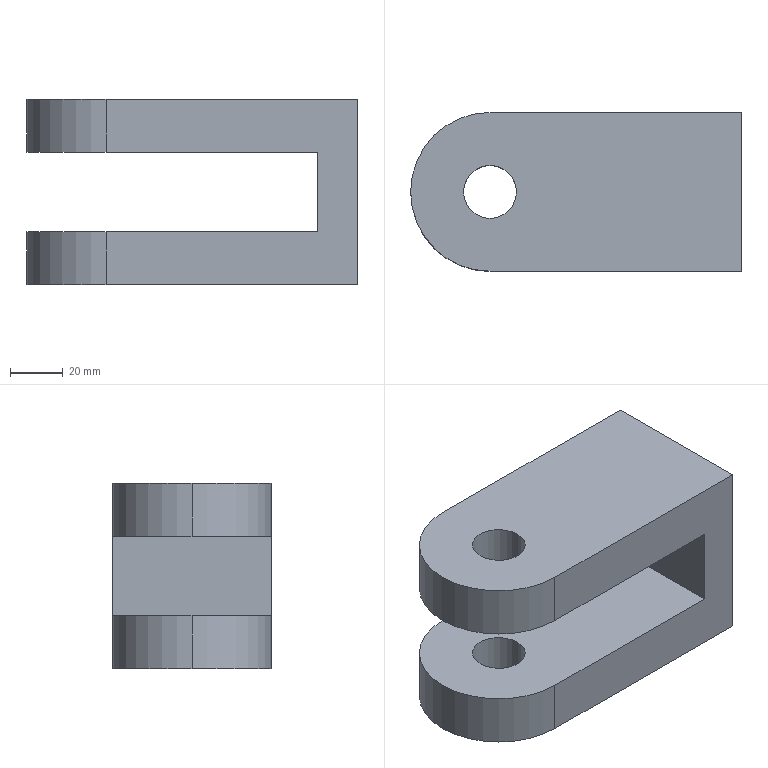Part | SolidWorks | features ICE 2, Extrusion 1, MirrorSolid 1 | 1 solid | 16 faces | box 125 x 60 x 70 mm | volume 298982 mm3 | cylinder 8 | plane 8 | commonest cylinder face diameters 20 x4 60 x4
STEP:
#1=CARTESIAN_POINT('',(-50.,0.,-50.));
#2=VERTEX_POINT('',#1);
#3=CARTESIAN_POINT('',(-30.,0.,-50.));
#4=VERTEX_POINT('',#3);
#5=CARTESIAN_POINT('',(-40.,0.,-50.));
#6=DIRECTION('',(0.,0.,-1.));
#7=DIRECTION('',(-1.,0.,0.));
#8=AXIS2_PLACEMENT_3D('',#5,#6,#7);
#9=CIRCLE('',#8,10.);
#10=EDGE_CURVE('',#2,#4,#9,.T.);
#11=ORIENTED_EDGE('',*,*,#10,.T.);
#12=CARTESIAN_POINT('',(-30.,0.,-30.));
#13=VERTEX_POINT('',#12);
#14=CARTESIAN_POINT('',(-30.,0.,-50.));
#15=DIRECTION('',(0.,0.,1.));
#16=VECTOR('',#15,1000.);
#17=LINE('',#14,#16);
#18=EDGE_CURVE('',#4,#13,#17,.T.);
#19=ORIENTED_EDGE('',*,*,#18,.T.);
#20=CARTESIAN_POINT('',(-50.,0.,-30.));
#21=VERTEX_POINT('',#20);
#22=CARTESIAN_POINT('',(-40.,0.,-30.));
#23=DIRECTION('',(0.,0.,-1.));
#24=DIRECTION('',(-1.,0.,0.));
#25=AXIS2_PLACEMENT_3D('',#22,#23,#24);
#26=CIRCLE('',#25,10.);
#27=EDGE_CURVE('',#21,#13,#26,.T.);
#28=ORIENTED_EDGE('',*,*,#27,.F.);
#29=CARTESIAN_POINT('',(-50.,0.,-50.));
#30=DIRECTION('',(0.,0.,1.));
#31=VECTOR('',#30,1000.);
#32=LINE('',#29,#31);
#33=EDGE_CURVE('',#2,#21,#32,.T.);
#34=ORIENTED_EDGE('',*,*,#33,.F.);
#35=EDGE_LOOP('',(#11,#19,#28,#34));
#36=FACE_OUTER_BOUND('',#35,.T.);
#37=CARTESIAN_POINT('',(-40.,0.,-50.));
#38=DIRECTION('',(0.,0.,1.));
#39=DIRECTION('',(-1.,0.,0.));
#40=AXIS2_PLACEMENT_3D('',#37,#38,#39);
#41=CYLINDRICAL_SURFACE('',#40,10.);
#42=ADVANCED_FACE('',(#36),#41,.F.);
#43=CARTESIAN_POINT('',(-40.,30.,-50.));
#44=VERTEX_POINT('',#43);
#45=CARTESIAN_POINT('',(-70.,0.,-50.));
#46=VERTEX_POINT('',#45);
#47=CARTESIAN_POINT('',(-40.,0.,-50.));
#48=DIRECTION('',(0.,0.,1.));
#49=DIRECTION('',(1.,0.,0.));
#50=AXIS2_PLACEMENT_3D('',#47,#48,#49);
#51=CIRCLE('',#50,30.);
#52=EDGE_CURVE('',#44,#46,#51,.T.);
#53=ORIENTED_EDGE('',*,*,#52,.T.);
#54=CARTESIAN_POINT('',(-70.,0.,-30.));
#55=VERTEX_POINT('',#54);
#56=CARTESIAN_POINT('',(-70.,0.,-50.));
#57=DIRECTION('',(0.,0.,1.));
#58=VECTOR('',#57,1000.);
#59=LINE('',#56,#58);
#60=EDGE_CURVE('',#46,#55,#59,.T.);
#61=ORIENTED_EDGE('',*,*,#60,.T.);
#62=CARTESIAN_POINT('',(-40.,30.,-30.));
#63=VERTEX_POINT('',#62);
#64=CARTESIAN_POINT('',(-40.,0.,-30.));
#65=DIRECTION('',(0.,0.,1.));
#66=DIRECTION('',(1.,0.,0.));
#67=AXIS2_PLACEMENT_3D('',#64,#65,#66);
#68=CIRCLE('',#67,30.);
#69=EDGE_CURVE('',#63,#55,#68,.T.);
#70=ORIENTED_EDGE('',*,*,#69,.F.);
#71=CARTESIAN_POINT('',(-40.,30.,-50.));
#72=DIRECTION('',(0.,0.,1.));
#73=VECTOR('',#72,1000.);
#74=LINE('',#71,#73);
#75=EDGE_CURVE('',#44,#63,#74,.T.);
#76=ORIENTED_EDGE('',*,*,#75,.F.);
#77=EDGE_LOOP('',(#53,#61,#70,#76));
#78=FACE_OUTER_BOUND('',#77,.T.);
#79=CARTESIAN_POINT('',(-40.,0.,-50.));
#80=DIRECTION('',(0.,0.,1.));
#81=DIRECTION('',(-1.,0.,0.));
#82=AXIS2_PLACEMENT_3D('',#79,#80,#81);
#83=CYLINDRICAL_SURFACE('',#82,30.);
#84=ADVANCED_FACE('',(#78),#83,.T.);
#85=CARTESIAN_POINT('',(-30.,0.,20.));
#86=VERTEX_POINT('',#85);
#87=CARTESIAN_POINT('',(-50.,0.,20.));
#88=VERTEX_POINT('',#87);
#89=CARTESIAN_POINT('',(-40.,0.,20.));
#90=DIRECTION('',(0.,0.,-1.));
#91=DIRECTION('',(-1.,0.,0.));
#92=AXIS2_PLACEMENT_3D('',#89,#90,#91);
#93=CIRCLE('',#92,10.);
#94=EDGE_CURVE('',#86,#88,#93,.T.);
#95=ORIENTED_EDGE('',*,*,#94,.F.);
#96=CARTESIAN_POINT('',(-30.,0.,0.));
#97=VERTEX_POINT('',#96);
#98=CARTESIAN_POINT('',(-30.,0.,20.));
#99=DIRECTION('',(0.,0.,-1.));
#100=VECTOR('',#99,1000.);
#101=LINE('',#98,#100);
#102=EDGE_CURVE('',#86,#97,#101,.T.);
#103=ORIENTED_EDGE('',*,*,#102,.T.);
#104=CARTESIAN_POINT('',(-50.,0.,0.));
#105=VERTEX_POINT('',#104);
#106=CARTESIAN_POINT('',(-40.,0.,0.));
#107=DIRECTION('',(0.,0.,-1.));
#108=DIRECTION('',(-1.,0.,0.));
#109=AXIS2_PLACEMENT_3D('',#106,#107,#108);
#110=CIRCLE('',#109,10.);
#111=EDGE_CURVE('',#97,#105,#110,.T.);
#112=ORIENTED_EDGE('',*,*,#111,.T.);
#113=CARTESIAN_POINT('',(-50.,0.,20.));
#114=DIRECTION('',(0.,0.,-1.));
#115=VECTOR('',#114,1000.);
#116=LINE('',#113,#115);
#117=EDGE_CURVE('',#88,#105,#116,.T.);
#118=ORIENTED_EDGE('',*,*,#117,.F.);
#119=EDGE_LOOP('',(#95,#103,#112,#118));
#120=FACE_OUTER_BOUND('',#119,.T.);
#121=CARTESIAN_POINT('',(-40.,0.,20.));
#122=DIRECTION('',(0.,0.,-1.));
#123=DIRECTION('',(-1.,0.,0.));
#124=AXIS2_PLACEMENT_3D('',#121,#122,#123);
#125=CYLINDRICAL_SURFACE('',#124,10.);
#126=ADVANCED_FACE('',(#120),#125,.F.);
#127=CARTESIAN_POINT('',(-70.,0.,20.));
#128=VERTEX_POINT('',#127);
#129=CARTESIAN_POINT('',(-40.,-30.,20.));
#130=VERTEX_POINT('',#129);
#131=CARTESIAN_POINT('',(-40.,0.,20.));
#132=DIRECTION('',(0.,0.,1.));
#133=DIRECTION('',(1.,0.,0.));
#134=AXIS2_PLACEMENT_3D('',#131,#132,#133);
#135=CIRCLE('',#134,30.);
#136=EDGE_CURVE('',#128,#130,#135,.T.);
#137=ORIENTED_EDGE('',*,*,#136,.F.);
#138=CARTESIAN_POINT('',(-70.,0.,0.));
#139=VERTEX_POINT('',#138);
#140=CARTESIAN_POINT('',(-70.,0.,20.));
#141=DIRECTION('',(0.,0.,-1.));
#142=VECTOR('',#141,1000.);
#143=LINE('',#140,#142);
#144=EDGE_CURVE('',#128,#139,#143,.T.);
#145=ORIENTED_EDGE('',*,*,#144,.T.);
#146=CARTESIAN_POINT('',(-40.,-30.,0.));
#147=VERTEX_POINT('',#146);
#148=CARTESIAN_POINT('',(-40.,0.,0.));
#149=DIRECTION('',(0.,0.,1.));
#150=DIRECTION('',(1.,0.,0.));
#151=AXIS2_PLACEMENT_3D('',#148,#149,#150);
#152=CIRCLE('',#151,30.);
#153=EDGE_CURVE('',#139,#147,#152,.T.);
#154=ORIENTED_EDGE('',*,*,#153,.T.);
#155=CARTESIAN_POINT('',(-40.,-30.,20.));
#156=DIRECTION('',(0.,0.,-1.));
#157=VECTOR('',#156,1000.);
#158=LINE('',#155,#157);
#159=EDGE_CURVE('',#130,#147,#158,.T.);
#160=ORIENTED_EDGE('',*,*,#159,.F.);
#161=EDGE_LOOP('',(#137,#145,#154,#160));
#162=FACE_OUTER_BOUND('',#161,.T.);
#163=CARTESIAN_POINT('',(-40.,0.,20.));
#164=DIRECTION('',(0.,0.,-1.));
#165=DIRECTION('',(-1.,0.,0.));
#166=AXIS2_PLACEMENT_3D('',#163,#164,#165);
#167=CYLINDRICAL_SURFACE('',#166,30.);
#168=ADVANCED_FACE('',(#162),#167,.T.);
#169=CARTESIAN_POINT('',(40.,30.,0.));
#170=VERTEX_POINT('',#169);
#171=CARTESIAN_POINT('',(-40.,30.,0.));
#172=VERTEX_POINT('',#171);
#173=CARTESIAN_POINT('',(-40.,30.,0.));
#174=DIRECTION('',(-1.,0.,0.));
#175=VECTOR('',#174,1000.);
#176=LINE('',#173,#175);
#177=EDGE_CURVE('',#170,#172,#176,.T.);
#178=ORIENTED_EDGE('',*,*,#177,.T.);
#179=CARTESIAN_POINT('',(-40.,30.,20.));
#180=VERTEX_POINT('',#179);
#181=CARTESIAN_POINT('',(-40.,30.,20.));
#182=DIRECTION('',(0.,0.,-1.));
#183=VECTOR('',#182,1000.);
#184=LINE('',#181,#183);
#185=EDGE_CURVE('',#180,#172,#184,.T.);
#186=ORIENTED_EDGE('',*,*,#185,.F.);
#187=CARTESIAN_POINT('',(55.,30.,20.));
#188=VERTEX_POINT('',#187);
#189=CARTESIAN_POINT('',(-40.,30.,20.));
#190=DIRECTION('',(-1.,0.,0.));
#191=VECTOR('',#190,1000.);
#192=LINE('',#189,#191);
#193=EDGE_CURVE('',#188,#180,#192,.T.);
#194=ORIENTED_EDGE('',*,*,#193,.F.);
#195=CARTESIAN_POINT('',(55.,30.,-50.));
#196=VERTEX_POINT('',#195);
#197=CARTESIAN_POINT('',(55.,30.,20.));
#198=DIRECTION('',(0.,0.,1.));
#199=VECTOR('',#198,1000.);
#200=LINE('',#197,#199);
#201=EDGE_CURVE('',#196,#188,#200,.T.);
#202=ORIENTED_EDGE('',*,*,#201,.F.);
#203=CARTESIAN_POINT('',(-40.,30.,-50.));
#204=DIRECTION('',(-1.,0.,0.));
#205=VECTOR('',#204,1000.);
#206=LINE('',#203,#205);
#207=EDGE_CURVE('',#196,#44,#206,.T.);
#208=ORIENTED_EDGE('',*,*,#207,.T.);
#209=ORIENTED_EDGE('',*,*,#75,.T.);
#210=CARTESIAN_POINT('',(40.,30.,-30.));
#211=VERTEX_POINT('',#210);
#212=CARTESIAN_POINT('',(-40.,30.,-30.));
#213=DIRECTION('',(-1.,0.,0.));
#214=VECTOR('',#213,1000.);
#215=LINE('',#212,#214);
#216=EDGE_CURVE('',#211,#63,#215,.T.);
#217=ORIENTED_EDGE('',*,*,#216,.F.);
#218=CARTESIAN_POINT('',(40.,30.,20.));
#219=DIRECTION('',(0.,0.,1.));
#220=VECTOR('',#219,1000.);
#221=LINE('',#218,#220);
#222=EDGE_CURVE('',#211,#170,#221,.T.);
#223=ORIENTED_EDGE('',*,*,#222,.T.);
#224=EDGE_LOOP('',(#178,#186,#194,#202,#208,#209,#217,#223));
#225=FACE_OUTER_BOUND('',#224,.T.);
#226=CARTESIAN_POINT('',(-40.,30.,20.));
#227=DIRECTION('',(0.,-1.,0.));
#228=DIRECTION('',(0.,0.,-1.));
#229=AXIS2_PLACEMENT_3D('',#226,#227,#228);
#230=PLANE('',#229);
#231=ADVANCED_FACE('',(#225),#230,.F.);
#232=ORIENTED_EDGE('',*,*,#144,.F.);
#233=CARTESIAN_POINT('',(-40.,0.,20.));
#234=DIRECTION('',(0.,0.,1.));
#235=DIRECTION('',(1.,0.,0.));
#236=AXIS2_PLACEMENT_3D('',#233,#234,#235);
#237=CIRCLE('',#236,30.);
#238=EDGE_CURVE('',#180,#128,#237,.T.);
#239=ORIENTED_EDGE('',*,*,#238,.F.);
#240=ORIENTED_EDGE('',*,*,#185,.T.);
#241=CARTESIAN_POINT('',(-40.,0.,0.));
#242=DIRECTION('',(0.,0.,1.));
#243=DIRECTION('',(1.,0.,0.));
#244=AXIS2_PLACEMENT_3D('',#241,#242,#243);
#245=CIRCLE('',#244,30.);
#246=EDGE_CURVE('',#172,#139,#245,.T.);
#247=ORIENTED_EDGE('',*,*,#246,.T.);
#248=EDGE_LOOP('',(#232,#239,#240,#247));
#249=FACE_OUTER_BOUND('',#248,.T.);
#250=CARTESIAN_POINT('',(-40.,0.,20.));
#251=DIRECTION('',(0.,0.,-1.));
#252=DIRECTION('',(-1.,0.,0.));
#253=AXIS2_PLACEMENT_3D('',#250,#251,#252);
#254=CYLINDRICAL_SURFACE('',#253,30.);
#255=ADVANCED_FACE('',(#249),#254,.T.);
#256=CARTESIAN_POINT('',(40.,-30.,0.));
#257=VERTEX_POINT('',#256);
#258=CARTESIAN_POINT('',(-40.,-30.,0.));
#259=DIRECTION('',(1.,0.,0.));
#260=VECTOR('',#259,1000.);
#261=LINE('',#258,#260);
#262=EDGE_CURVE('',#147,#257,#261,.T.);
#263=ORIENTED_EDGE('',*,*,#262,.T.);
#264=CARTESIAN_POINT('',(40.,-30.,-30.));
#265=VERTEX_POINT('',#264);
#266=CARTESIAN_POINT('',(40.,-30.,20.));
#267=DIRECTION('',(0.,0.,-1.));
#268=VECTOR('',#267,1000.);
#269=LINE('',#266,#268);
#270=EDGE_CURVE('',#257,#265,#269,.T.);
#271=ORIENTED_EDGE('',*,*,#270,.T.);
#272=CARTESIAN_POINT('',(-40.,-30.,-30.));
#273=VERTEX_POINT('',#272);
#274=CARTESIAN_POINT('',(-40.,-30.,-30.));
#275=DIRECTION('',(1.,0.,0.));
#276=VECTOR('',#275,1000.);
#277=LINE('',#274,#276);
#278=EDGE_CURVE('',#273,#265,#277,.T.);
#279=ORIENTED_EDGE('',*,*,#278,.F.);
#280=CARTESIAN_POINT('',(-40.,-30.,-50.));
#281=VERTEX_POINT('',#280);
#282=CARTESIAN_POINT('',(-40.,-30.,-50.));
#283=DIRECTION('',(0.,0.,1.));
#284=VECTOR('',#283,1000.);
#285=LINE('',#282,#284);
#286=EDGE_CURVE('',#281,#273,#285,.T.);
#287=ORIENTED_EDGE('',*,*,#286,.F.);
#288=CARTESIAN_POINT('',(55.,-30.,-50.));
#289=VERTEX_POINT('',#288);
#290=CARTESIAN_POINT('',(-40.,-30.,-50.));
#291=DIRECTION('',(1.,0.,0.));
#292=VECTOR('',#291,1000.);
#293=LINE('',#290,#292);
#294=EDGE_CURVE('',#281,#289,#293,.T.);
#295=ORIENTED_EDGE('',*,*,#294,.T.);
#296=CARTESIAN_POINT('',(55.,-30.,20.));
#297=VERTEX_POINT('',#296);
#298=CARTESIAN_POINT('',(55.,-30.,20.));
#299=DIRECTION('',(0.,0.,-1.));
#300=VECTOR('',#299,1000.);
#301=LINE('',#298,#300);
#302=EDGE_CURVE('',#297,#289,#301,.T.);
#303=ORIENTED_EDGE('',*,*,#302,.F.);
#304=CARTESIAN_POINT('',(-40.,-30.,20.));
#305=DIRECTION('',(1.,0.,0.));
#306=VECTOR('',#305,1000.);
#307=LINE('',#304,#306);
#308=EDGE_CURVE('',#130,#297,#307,.T.);
#309=ORIENTED_EDGE('',*,*,#308,.F.);
#310=ORIENTED_EDGE('',*,*,#159,.T.);
#311=EDGE_LOOP('',(#263,#271,#279,#287,#295,#303,#309,#310));
#312=FACE_OUTER_BOUND('',#311,.T.);
#313=CARTESIAN_POINT('',(-40.,-30.,20.));
#314=DIRECTION('',(0.,1.,0.));
#315=DIRECTION('',(0.,0.,1.));
#316=AXIS2_PLACEMENT_3D('',#313,#314,#315);
#317=PLANE('',#316);
#318=ADVANCED_FACE('',(#312),#317,.F.);
#319=CARTESIAN_POINT('',(-40.,0.,20.));
#320=DIRECTION('',(0.,0.,-1.));
#321=DIRECTION('',(-1.,0.,0.));
#322=AXIS2_PLACEMENT_3D('',#319,#320,#321);
#323=CIRCLE('',#322,10.);
#324=EDGE_CURVE('',#88,#86,#323,.T.);
#325=ORIENTED_EDGE('',*,*,#324,.T.);
#326=ORIENTED_EDGE('',*,*,#94,.T.);
#327=EDGE_LOOP('',(#325,#326));
#328=FACE_BOUND('',#327,.T.);
#329=ORIENTED_EDGE('',*,*,#308,.T.);
#330=CARTESIAN_POINT('',(55.,-30.,20.));
#331=DIRECTION('',(0.,-1.,0.));
#332=VECTOR('',#331,1000.);
#333=LINE('',#330,#332);
#334=EDGE_CURVE('',#188,#297,#333,.T.);
#335=ORIENTED_EDGE('',*,*,#334,.F.);
#336=ORIENTED_EDGE('',*,*,#193,.T.);
#337=ORIENTED_EDGE('',*,*,#238,.T.);
#338=ORIENTED_EDGE('',*,*,#136,.T.);
#339=EDGE_LOOP('',(#329,#335,#336,#337,#338));
#340=FACE_OUTER_BOUND('',#339,.T.);
#341=CARTESIAN_POINT('',(-40.,0.,20.));
#342=DIRECTION('',(0.,0.,1.));
#343=DIRECTION('',(1.,0.,0.));
#344=AXIS2_PLACEMENT_3D('',#341,#342,#343);
#345=PLANE('',#344);
#346=ADVANCED_FACE('',(#328,#340),#345,.T.);
#347=CARTESIAN_POINT('',(-40.,0.,0.));
#348=DIRECTION('',(0.,0.,-1.));
#349=DIRECTION('',(-1.,0.,0.));
#350=AXIS2_PLACEMENT_3D('',#347,#348,#349);
#351=CIRCLE('',#350,10.);
#352=EDGE_CURVE('',#105,#97,#351,.T.);
#353=ORIENTED_EDGE('',*,*,#352,.F.);
#354=ORIENTED_EDGE('',*,*,#111,.F.);
#355=EDGE_LOOP('',(#353,#354));
#356=FACE_BOUND('',#355,.T.);
#357=CARTESIAN_POINT('',(40.,30.,0.));
#358=DIRECTION('',(0.,1.,0.));
#359=VECTOR('',#358,1000.);
#360=LINE('',#357,#359);
#361=EDGE_CURVE('',#257,#170,#360,.T.);
#362=ORIENTED_EDGE('',*,*,#361,.F.);
#363=ORIENTED_EDGE('',*,*,#262,.F.);
#364=ORIENTED_EDGE('',*,*,#153,.F.);
#365=ORIENTED_EDGE('',*,*,#246,.F.);
#366=ORIENTED_EDGE('',*,*,#177,.F.);
#367=EDGE_LOOP('',(#362,#363,#364,#365,#366));
#368=FACE_OUTER_BOUND('',#367,.T.);
#369=CARTESIAN_POINT('',(-40.,0.,0.));
#370=DIRECTION('',(0.,0.,1.));
#371=DIRECTION('',(1.,0.,0.));
#372=AXIS2_PLACEMENT_3D('',#369,#370,#371);
#373=PLANE('',#372);
#374=ADVANCED_FACE('',(#356,#368),#373,.F.);
#375=ORIENTED_EDGE('',*,*,#102,.F.);
#376=ORIENTED_EDGE('',*,*,#324,.F.);
#377=ORIENTED_EDGE('',*,*,#117,.T.);
#378=ORIENTED_EDGE('',*,*,#352,.T.);
#379=EDGE_LOOP('',(#375,#376,#377,#378));
#380=FACE_OUTER_BOUND('',#379,.T.);
#381=CARTESIAN_POINT('',(-40.,0.,20.));
#382=DIRECTION('',(0.,0.,-1.));
#383=DIRECTION('',(-1.,0.,0.));
#384=AXIS2_PLACEMENT_3D('',#381,#382,#383);
#385=CYLINDRICAL_SURFACE('',#384,10.);
#386=ADVANCED_FACE('',(#380),#385,.F.);
#387=ORIENTED_EDGE('',*,*,#270,.F.);
#388=ORIENTED_EDGE('',*,*,#361,.T.);
#389=ORIENTED_EDGE('',*,*,#222,.F.);
#390=CARTESIAN_POINT('',(40.,30.,-30.));
#391=DIRECTION('',(0.,1.,0.));
#392=VECTOR('',#391,1000.);
#393=LINE('',#390,#392);
#394=EDGE_CURVE('',#265,#211,#393,.T.);
#395=ORIENTED_EDGE('',*,*,#394,.F.);
#396=EDGE_LOOP('',(#387,#388,#389,#395));
#397=FACE_OUTER_BOUND('',#396,.T.);
#398=CARTESIAN_POINT('',(40.,0.,0.));
#399=DIRECTION('',(1.,0.,0.));
#400=DIRECTION('',(0.,0.,-1.));
#401=AXIS2_PLACEMENT_3D('',#398,#399,#400);
#402=PLANE('',#401);
#403=ADVANCED_FACE('',(#397),#402,.F.);
#404=ORIENTED_EDGE('',*,*,#302,.T.);
#405=CARTESIAN_POINT('',(55.,-30.,-50.));
#406=DIRECTION('',(0.,-1.,0.));
#407=VECTOR('',#406,1000.);
#408=LINE('',#405,#407);
#409=EDGE_CURVE('',#196,#289,#408,.T.);
#410=ORIENTED_EDGE('',*,*,#409,.F.);
#411=ORIENTED_EDGE('',*,*,#201,.T.);
#412=ORIENTED_EDGE('',*,*,#334,.T.);
#413=EDGE_LOOP('',(#404,#410,#411,#412));
#414=FACE_OUTER_BOUND('',#413,.T.);
#415=CARTESIAN_POINT('',(55.,0.,0.));
#416=DIRECTION('',(1.,0.,0.));
#417=DIRECTION('',(0.,0.,-1.));
#418=AXIS2_PLACEMENT_3D('',#415,#416,#417);
#419=PLANE('',#418);
#420=ADVANCED_FACE('',(#414),#419,.T.);
#421=ORIENTED_EDGE('',*,*,#60,.F.);
#422=CARTESIAN_POINT('',(-40.,0.,-50.));
#423=DIRECTION('',(0.,0.,1.));
#424=DIRECTION('',(1.,0.,0.));
#425=AXIS2_PLACEMENT_3D('',#422,#423,#424);
#426=CIRCLE('',#425,30.);
#427=EDGE_CURVE('',#46,#281,#426,.T.);
#428=ORIENTED_EDGE('',*,*,#427,.T.);
#429=ORIENTED_EDGE('',*,*,#286,.T.);
#430=CARTESIAN_POINT('',(-40.,0.,-30.));
#431=DIRECTION('',(0.,0.,1.));
#432=DIRECTION('',(1.,0.,0.));
#433=AXIS2_PLACEMENT_3D('',#430,#431,#432);
#434=CIRCLE('',#433,30.);
#435=EDGE_CURVE('',#55,#273,#434,.T.);
#436=ORIENTED_EDGE('',*,*,#435,.F.);
#437=EDGE_LOOP('',(#421,#428,#429,#436));
#438=FACE_OUTER_BOUND('',#437,.T.);
#439=CARTESIAN_POINT('',(-40.,0.,-50.));
#440=DIRECTION('',(0.,0.,1.));
#441=DIRECTION('',(-1.,0.,0.));
#442=AXIS2_PLACEMENT_3D('',#439,#440,#441);
#443=CYLINDRICAL_SURFACE('',#442,30.);
#444=ADVANCED_FACE('',(#438),#443,.T.);
#445=ORIENTED_EDGE('',*,*,#10,.F.);
#446=CARTESIAN_POINT('',(-40.,0.,-50.));
#447=DIRECTION('',(0.,0.,-1.));
#448=DIRECTION('',(-1.,0.,0.));
#449=AXIS2_PLACEMENT_3D('',#446,#447,#448);
#450=CIRCLE('',#449,10.);
#451=EDGE_CURVE('',#4,#2,#450,.T.);
#452=ORIENTED_EDGE('',*,*,#451,.F.);
#453=EDGE_LOOP('',(#445,#452));
#454=FACE_BOUND('',#453,.T.);
#455=ORIENTED_EDGE('',*,*,#294,.F.);
#456=ORIENTED_EDGE('',*,*,#427,.F.);
#457=ORIENTED_EDGE('',*,*,#52,.F.);
#458=ORIENTED_EDGE('',*,*,#207,.F.);
#459=ORIENTED_EDGE('',*,*,#409,.T.);
#460=EDGE_LOOP('',(#455,#456,#457,#458,#459));
#461=FACE_OUTER_BOUND('',#460,.T.);
#462=CARTESIAN_POINT('',(-40.,0.,-50.));
#463=DIRECTION('',(0.,0.,-1.));
#464=DIRECTION('',(1.,0.,0.));
#465=AXIS2_PLACEMENT_3D('',#462,#463,#464);
#466=PLANE('',#465);
#467=ADVANCED_FACE('',(#454,#461),#466,.T.);
#468=ORIENTED_EDGE('',*,*,#27,.T.);
#469=CARTESIAN_POINT('',(-40.,0.,-30.));
#470=DIRECTION('',(0.,0.,-1.));
#471=DIRECTION('',(-1.,0.,0.));
#472=AXIS2_PLACEMENT_3D('',#469,#470,#471);
#473=CIRCLE('',#472,10.);
#474=EDGE_CURVE('',#13,#21,#473,.T.);
#475=ORIENTED_EDGE('',*,*,#474,.T.);
#476=EDGE_LOOP('',(#468,#475));
#477=FACE_BOUND('',#476,.T.);
#478=ORIENTED_EDGE('',*,*,#394,.T.);
#479=ORIENTED_EDGE('',*,*,#216,.T.);
#480=ORIENTED_EDGE('',*,*,#69,.T.);
#481=ORIENTED_EDGE('',*,*,#435,.T.);
#482=ORIENTED_EDGE('',*,*,#278,.T.);
#483=EDGE_LOOP('',(#478,#479,#480,#481,#482));
#484=FACE_OUTER_BOUND('',#483,.T.);
#485=CARTESIAN_POINT('',(-40.,0.,-30.));
#486=DIRECTION('',(0.,0.,-1.));
#487=DIRECTION('',(1.,0.,0.));
#488=AXIS2_PLACEMENT_3D('',#485,#486,#487);
#489=PLANE('',#488);
#490=ADVANCED_FACE('',(#477,#484),#489,.F.);
#491=ORIENTED_EDGE('',*,*,#18,.F.);
#492=ORIENTED_EDGE('',*,*,#451,.T.);
#493=ORIENTED_EDGE('',*,*,#33,.T.);
#494=ORIENTED_EDGE('',*,*,#474,.F.);
#495=EDGE_LOOP('',(#491,#492,#493,#494));
#496=FACE_OUTER_BOUND('',#495,.T.);
#497=CARTESIAN_POINT('',(-40.,0.,-50.));
#498=DIRECTION('',(0.,0.,1.));
#499=DIRECTION('',(-1.,0.,0.));
#500=AXIS2_PLACEMENT_3D('',#497,#498,#499);
#501=CYLINDRICAL_SURFACE('',#500,10.);
#502=ADVANCED_FACE('',(#496),#501,.F.);
#503=CLOSED_SHELL('',(#42,#84,#126,#168,#231,#255,#318,#346,#374,#386,#403,#420,#444,#467,#490,#502));
#504=MANIFOLD_SOLID_BREP('',#503);
#505=CARTESIAN_POINT('',(0.,0.,0.));
#506=DIRECTION('',(0.,0.,1.));
#507=DIRECTION('',(1.,0.,0.));
#508=AXIS2_PLACEMENT_3D('',#505,#506,#507);
#509=(LENGTH_UNIT()NAMED_UNIT(*)SI_UNIT(.MILLI.,.METRE.));
#510=UNCERTAINTY_MEASURE_WITH_UNIT(LENGTH_MEASURE(0.00001),#509,'','');
#511=(NAMED_UNIT(*)PLANE_ANGLE_UNIT()SI_UNIT($,.RADIAN.));
#512=(NAMED_UNIT(*)SI_UNIT($,.STERADIAN.)SOLID_ANGLE_UNIT());
#513=(GEOMETRIC_REPRESENTATION_CONTEXT(3)GLOBAL_UNCERTAINTY_ASSIGNED_CONTEXT((#510))GLOBAL_UNIT_ASSIGNED_CONTEXT((#509,#511,#512))REPRESENTATION_CONTEXT('',''));
#514=ADVANCED_BREP_SHAPE_REPRESENTATION('',(#504,#508),#513);